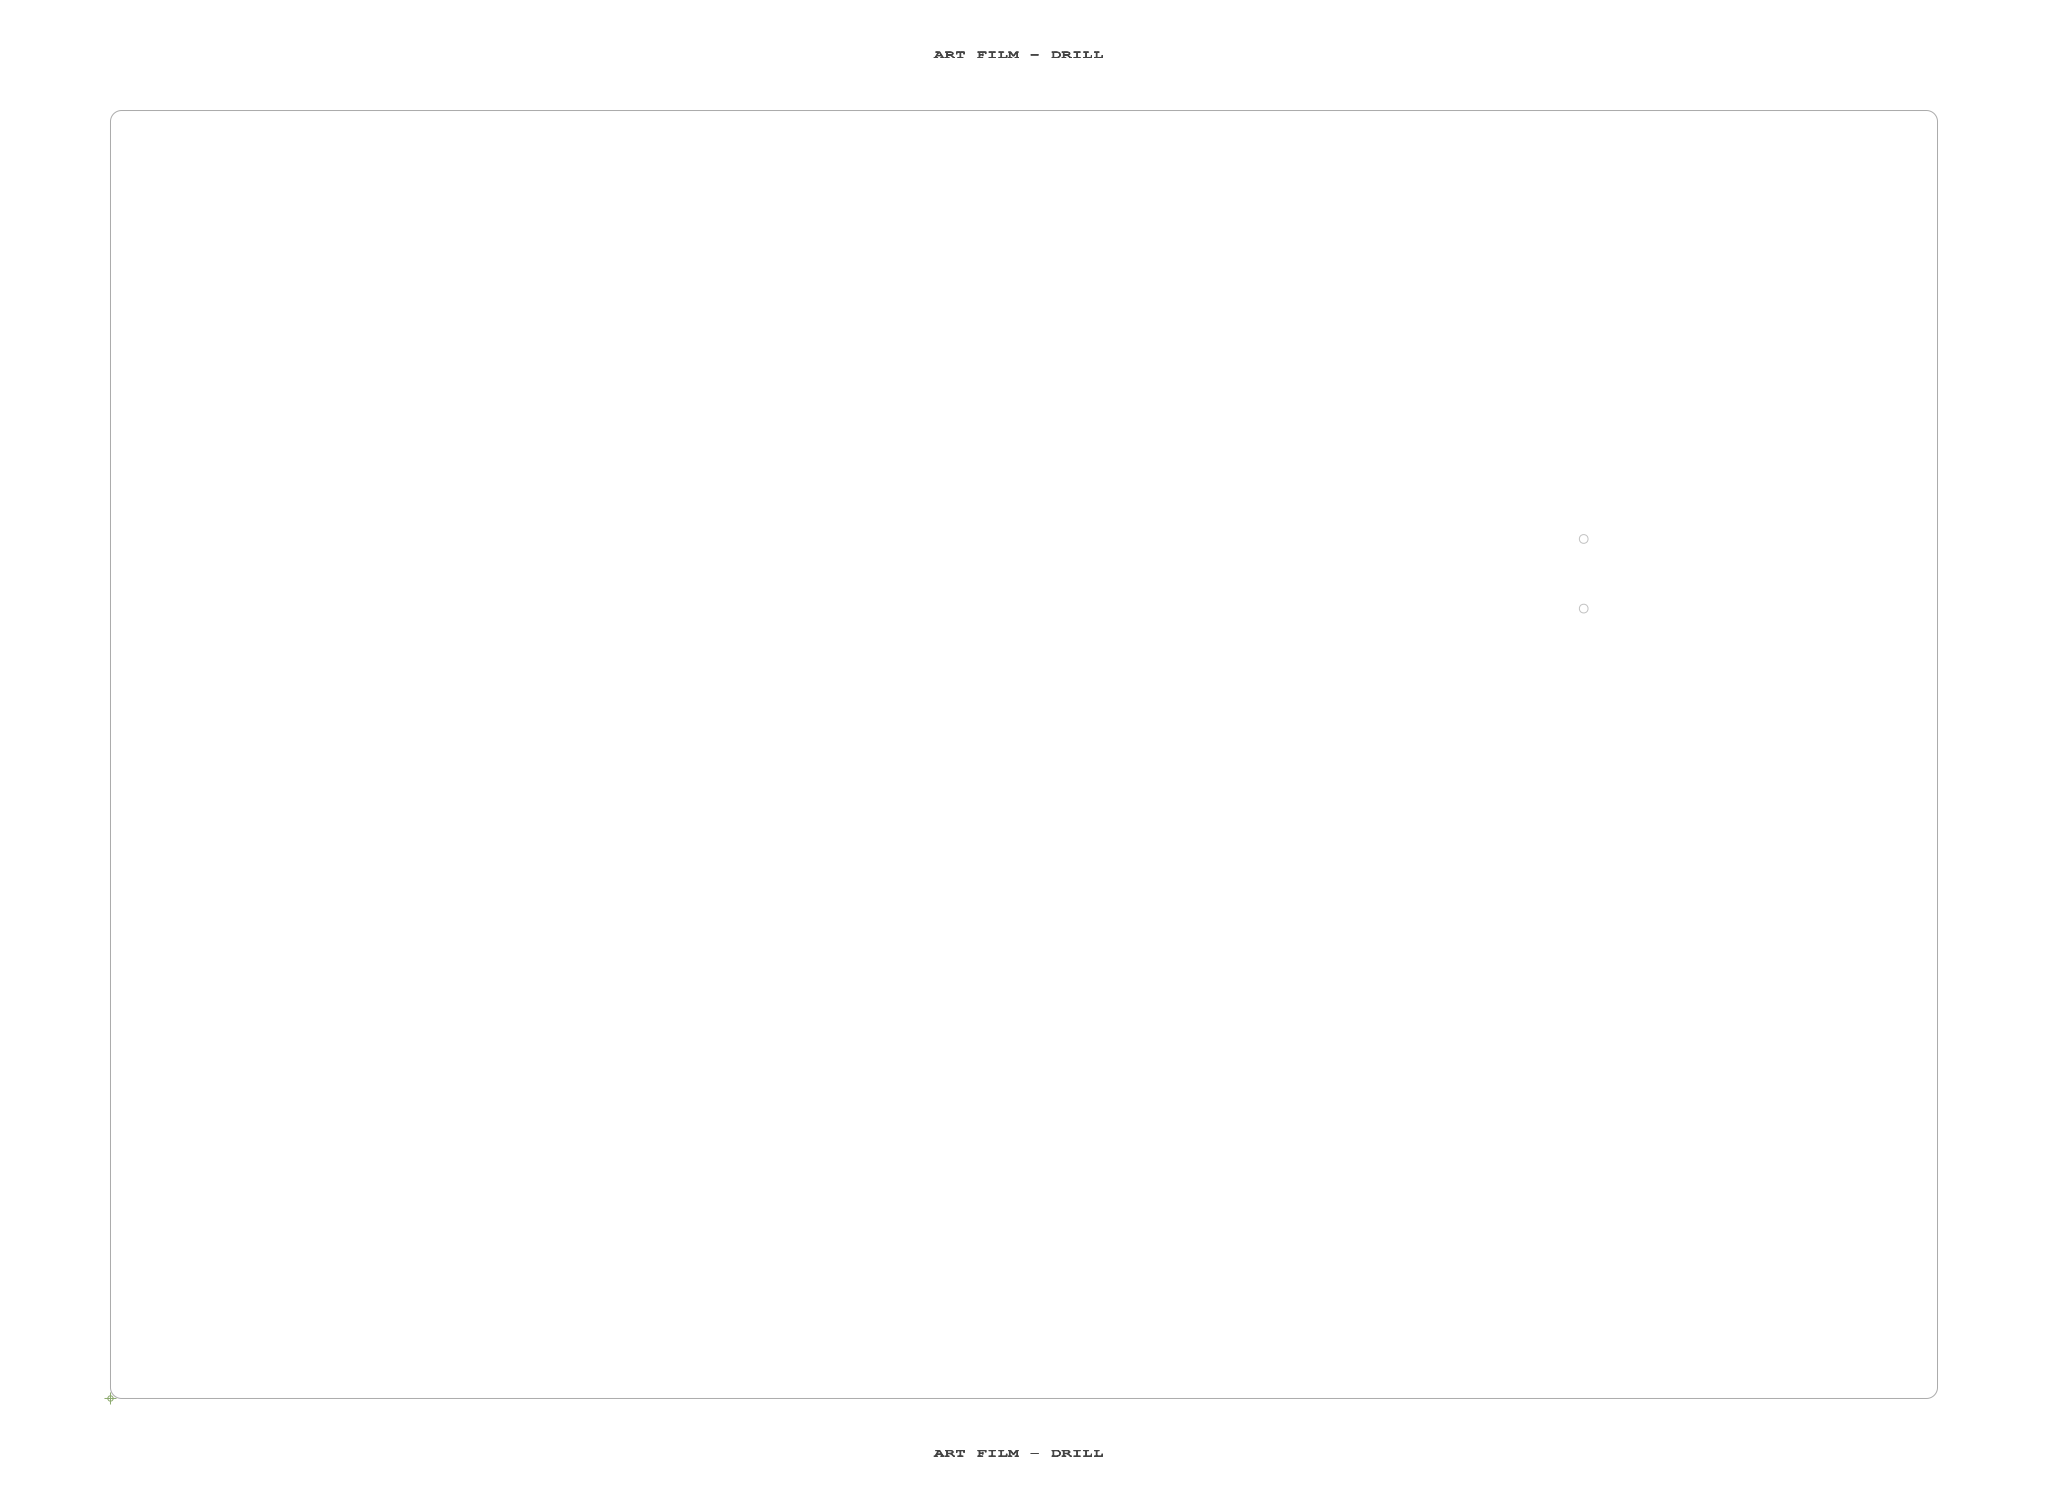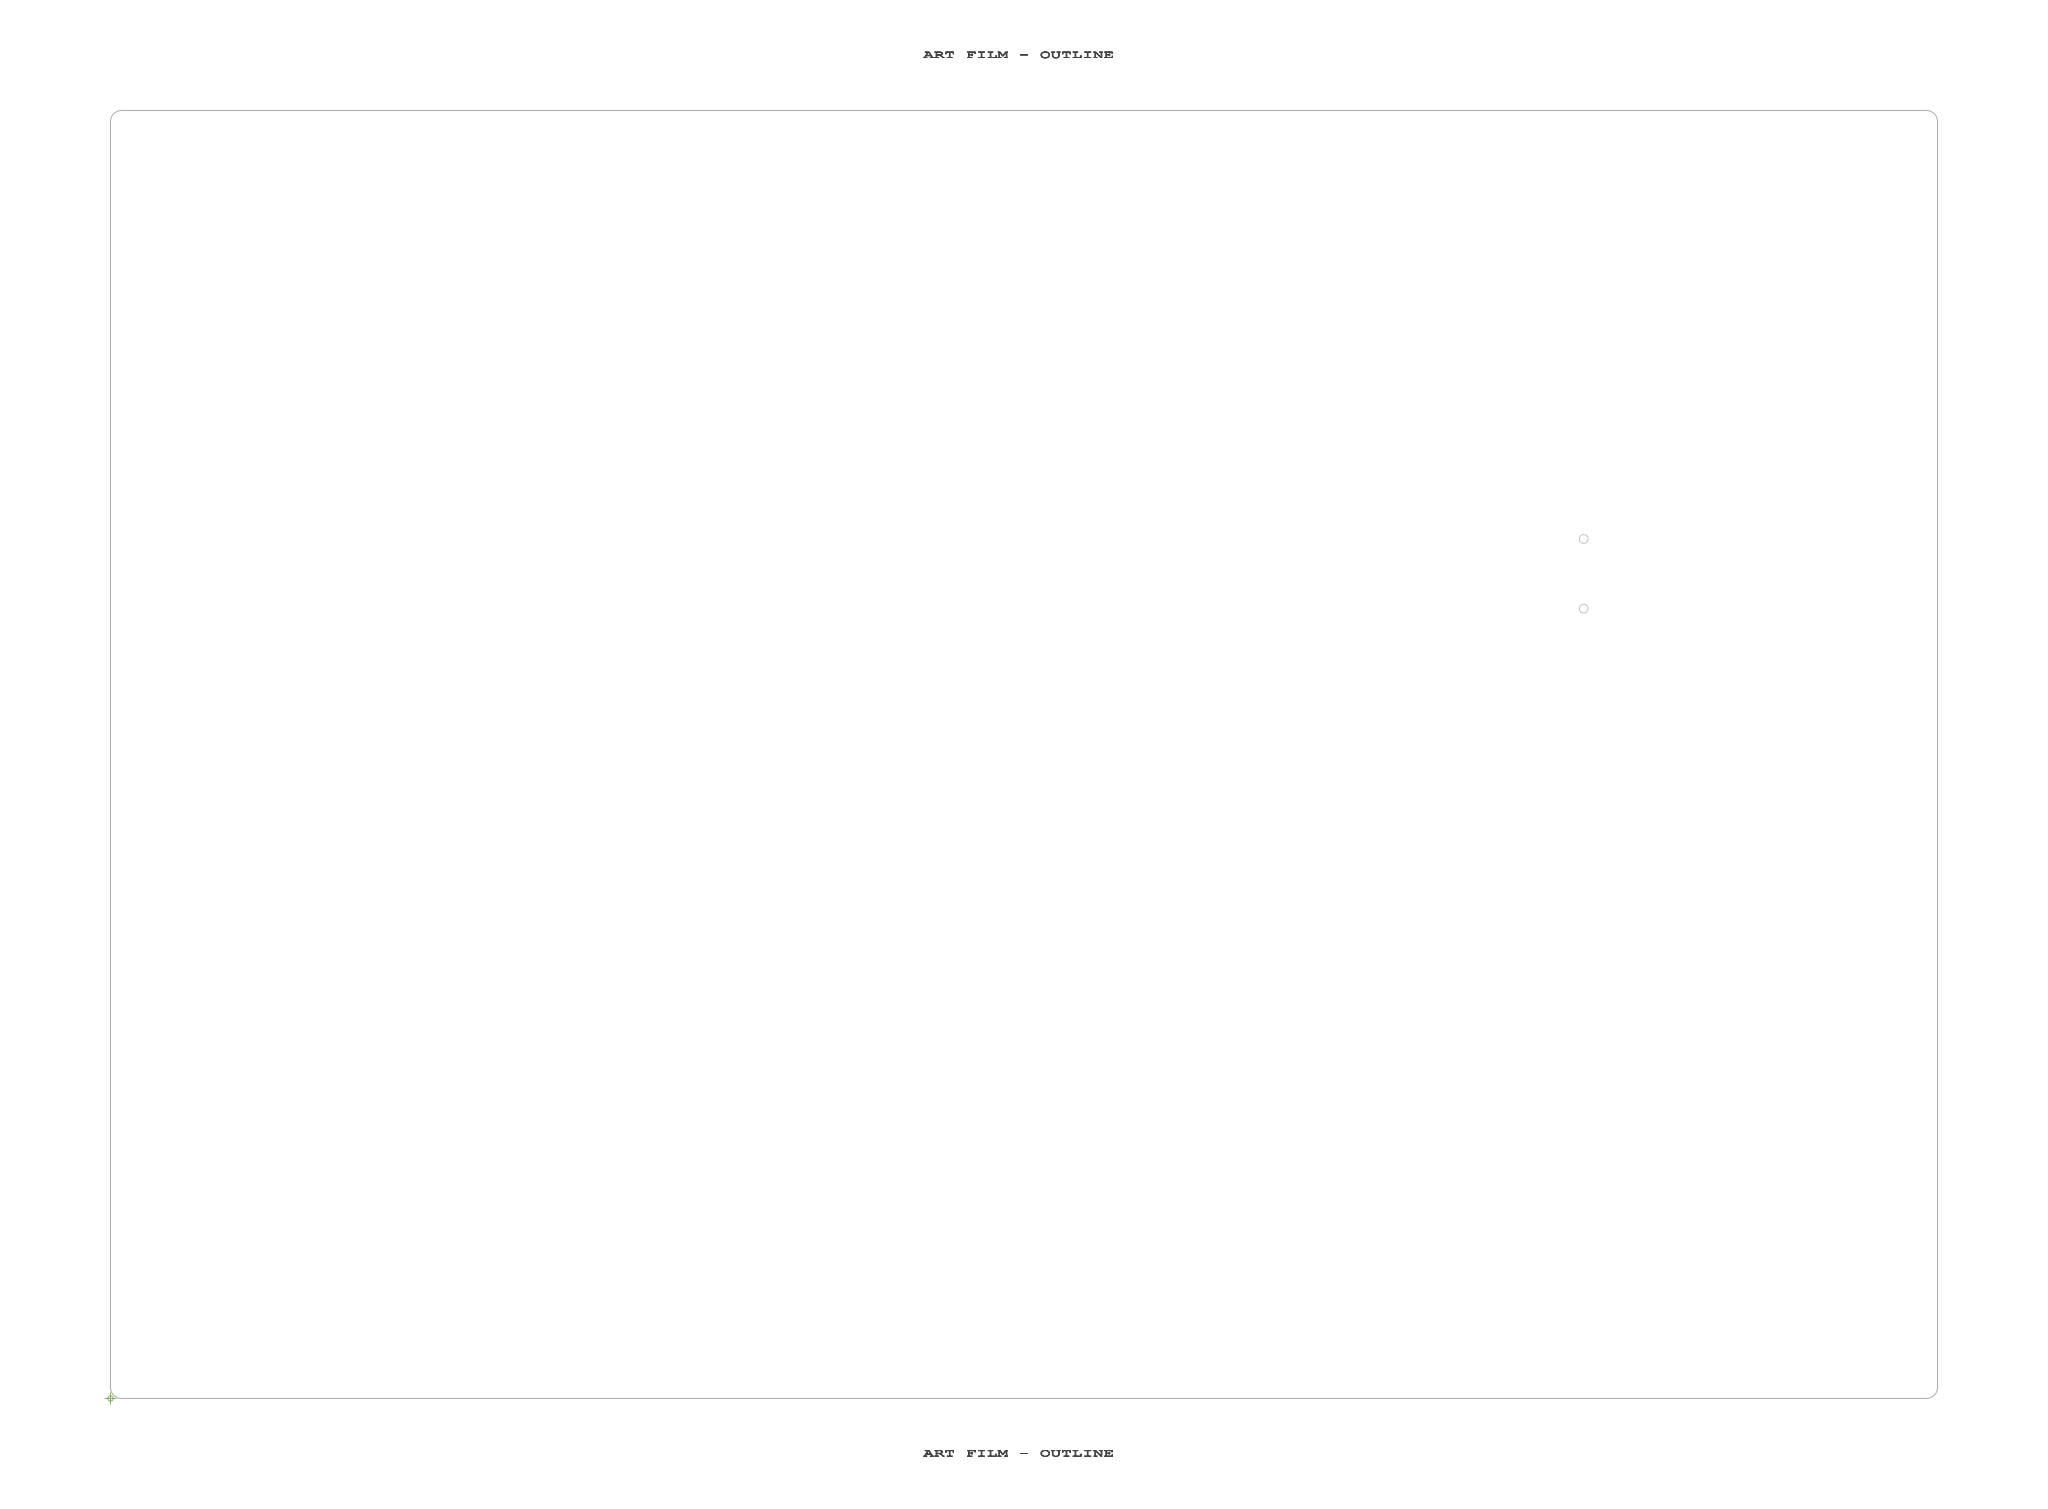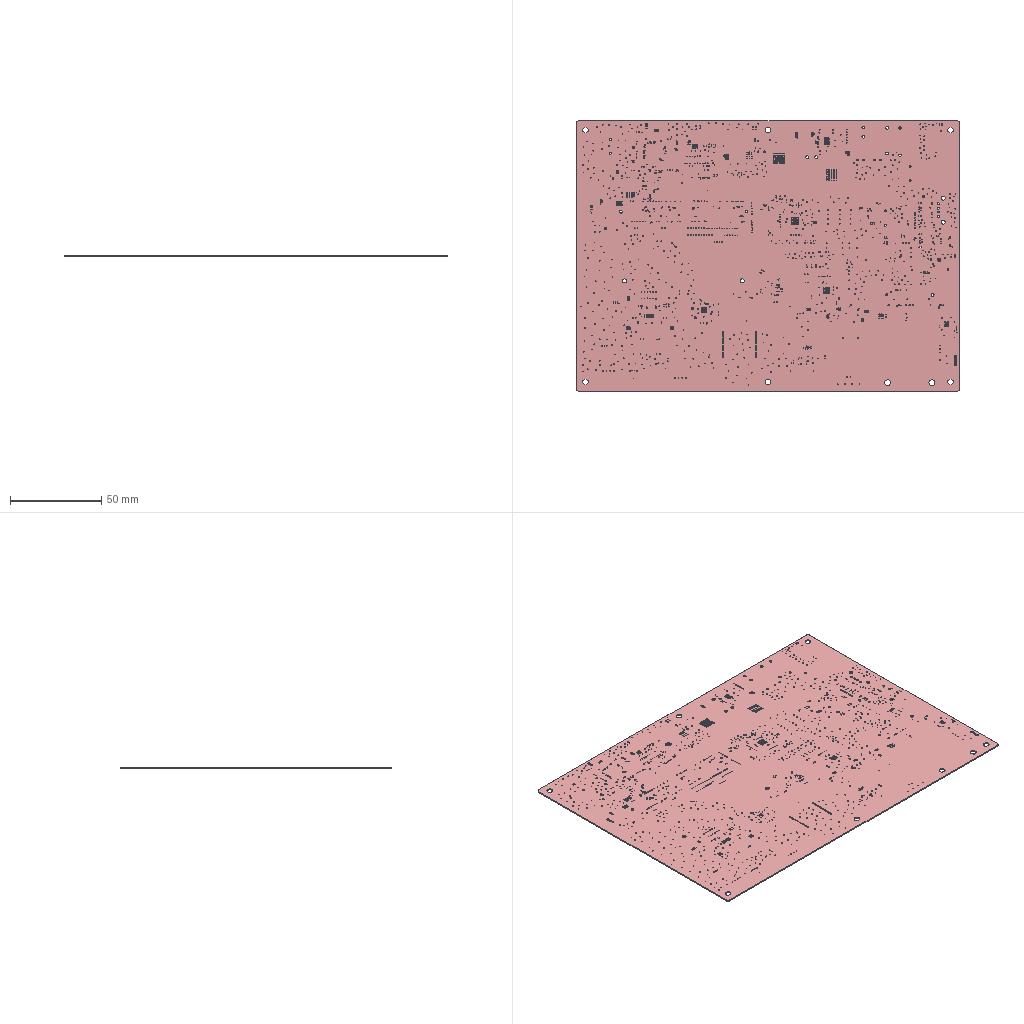Circuit board layout | Cadence Allegro | box 210 x 148 x 0.7 mm
Layer stack:
# Cadence Allegro layer stack of  (unit mm; from the constraint file cross-section; dielectric type: 0 not recorded (Allegro does not mark core vs prepreg), 3 surface material)
index,name,kind,layer,copper_thickness_mm,dielectric_type,dielectric_thickness_mm,dielectric_material,dielectric_constant
0,Top Surface,other,,,,,,
1,TOP,copper,TOP,0.0305,,,,
2,Dielectric1,dielectric,,,0,0.2032,FR-4,4.5
3,GND2,copper,GND2,0.0305,,,,
4,Dielectric2,dielectric,,,0,0.2032,FR-4,4.5
5,VCC3,copper,VCC3,0.0305,,,,
6,Dielectric3,dielectric,,,0,0.2032,FR-4,4.5
7,BOTTOM,copper,BOTTOM,0.0305,,,,
8,Bottom Surface,other,,,,,,
# drill layer pairs: low layer,high layer
drill_pair,TOP,BOTTOM
Part placement, first 550 of 616 lines:
REFDES,COMP_VALUE,SYM_NAME,SYM_X,SYM_Y,SYM_ROTATE,SYM_MIRROR
BT1,3V BAT,BAT600,731.008,5280.740,180.000,NO
C1,0.1uF/275V,C_18X6L,6981.850,5380.748,270.000,NO
C2,100nF,C0603,6496.929,4878.504,0.000,YES
C3,100nF,C0603,4264.664,5392.967,270.000,NO
C4,100nF,C0603,5492.165,5274.055,0.000,YES
C5,100nF,C0603,5766.479,5354.193,0.000,NO
C6,1uF,C0603,5278.819,5296.654,270.000,YES
C7,1uF,C0603,5765.731,5530.531,0.000,YES
C8,330pF,C0603,5767.402,5586.993,0.000,NO
C9,100nF,C0603,5768.303,5644.372,0.000,NO
C10,10nF,C0603,5462.622,5634.250,0.000,NO
C11,100nF,C0603,4031.414,5277.712,0.000,YES
C12,10uF/16V,C1206,3986.867,5314.380,180.000,NO
C13,2.2nF,C0603,5462.898,5566.801,0.000,NO
C14,1uF,C0603,5279.173,5424.528,90.000,YES
C15,10uF/16V,C1206,2817.520,5683.311,180.000,NO
C16,100nF,C0603,2558.740,5380.433,270.000,YES
C17,100nF,C0603,3352.205,5043.366,180.000,YES
C18,10uF/16V,C1206,3708.783,5592.795,90.000,NO
C19,10uF/16V,C1206,4892.301,1037.077,270.000,NO
C20,100nF,C0603,8083.170,1525.692,270.000,YES
C21,1nF,C0603,3502.319,4768.850,270.000,NO
C22,100nF,C0603,5241.942,1678.011,0.000,YES
C23,100nF,C0603,8202.820,1450.328,90.000,NO
C24,10uF/16V,C1206,7896.426,1719.824,90.000,NO
C25,100nF,C0603,3330.071,4721.878,180.000,YES
C26,100nF,C0603,8156.690,1222.130,90.000,YES
C27,100nF,C0603,4826.647,1609.621,90.000,NO
C28,100nF,C0603,5423.307,2711.417,90.000,YES
C29,100nF,C0603,5511.377,2212.857,270.000,YES
C30,22pF/50V,C0603,4973.224,2384.386,0.000,YES
C31,100nF,C0603,706.654,4602.992,0.000,NO
C32,22pF/50V,C0603,4962.673,2473.283,180.000,YES
C33,1nF,C0603,832.638,4595.157,270.000,YES
C34,100nF,C0603,937.205,4611.535,90.000,YES
C35,1uF/16V,C0603,5141.297,2057.270,180.000,NO
C36,1uF/16V,C0603,5586.850,2194.449,90.000,NO
C37,100nF,C0603,5296.181,2405.748,270.000,YES
C38,100nF,C0603,1123.346,4574.764,180.000,YES
C39,100nF,C0603,1465.315,4392.087,0.000,YES
C40,100nF,C0603,1485.709,4491.969,180.000,YES
C41,10uF/6.3V,C0805,1745.787,4651.279,0.000,NO
C42,100nF,C0603,1742.637,4568.602,0.000,NO
C43,10uF/6.3V,C0805,5154.232,3379.386,270.000,NO
C44,100nF,C0603,5037.118,3353.618,0.000,NO
C45,100nF,C0603,4741.547,3437.087,270.000,NO
C46,22pF/50V,C0603,5004.016,3745.902,180.000,YES
C47,100nF,C0603,4684.720,3436.811,270.000,NO
C48,100nF,C0603,4704.346,3554.295,0.000,YES
C49,100nF,C0603,4832.500,3736.449,270.000,YES
C50,100nF,C0603,4840.000,3875.000,180.000,YES
C51,22pF/50V,C0603,5015.236,3655.579,0.000,YES
C52,100nF,C0603,5159.031,3880.701,180.000,YES
C53,1uF/16V,C0603,5021.559,3880.874,0.000,NO
C54,100nF,C0603,4720.409,3790.437,0.000,YES
C55,100nF,C0603,4830.224,3604.929,90.000,YES
C56,10uF/6.3V,C0805,4690.162,4062.890,180.000,NO
C57,100nF,C0603,3620.700,2111.190,90.000,NO
C58,1nF/2kV,C1206,8054.163,483.534,0.000,YES
C59,100nF,C0603,3863.570,2117.570,270.000,NO
C60,100nF,C0603,3425.640,2116.160,270.000,NO
C61,100nF,C0603,2841.681,1765.520,90.000,YES
C62,100nF,C0603,2761.866,1843.043,0.000,YES
C63,4.7uF/16V,C0603,2531.024,1674.752,180.000,NO
C64,4.7uF/16V,C0603,2681.594,1535.354,270.000,NO
C65,4.7uF/16V,C0603,2821.295,1535.118,270.000,NO
C66,100nF,C0603,805.075,1990.827,90.000,NO
C67,4.7uF/16V,C0603,2741.634,1535.354,270.000,NO
C68,4.7uF/16V,C0603,2993.740,1643.618,0.000,NO
C69,1uF/16V,C0603,2989.008,1760.673,180.000,NO
C70,1nF,C0603,1945.232,1503.882,270.000,YES
C71,100nF,C0603,1878.988,1503.898,270.000,YES
C72,1uF/16V,C0603,1663.343,1897.094,270.000,NO
C73,220nF,C0603,1792.870,1359.024,270.000,NO
C74,330pF,C0603,1789.287,1181.031,270.000,NO
C75,1nF,C0603,1789.413,1049.197,90.000,NO
C76,1nF/50V,C0603,1723.972,1898.354,270.000,NO
C77,1uF/16V,C0603,1609.091,1897.488,270.000,NO
C78,4.7uF/16V,C0603,1719.201,2068.079,270.000,YES
C79,220nF,C0603,1623.618,1355.323,270.000,NO
C80,1nF,C0603,1734.728,1048.094,90.000,NO
C81,330pF,C0603,1735.823,1181.031,270.000,NO
C82,220nF,C0603,1567.831,1355.323,270.000,NO
C83,330pF,C0603,1450.469,1185.756,270.000,NO
C84,1nF,C0603,1452.051,1054.276,90.000,NO
C85,1uF/16V,C0603,1513.264,1896.780,270.000,NO
C86,1uF/16V,C0603,1457.122,1896.543,270.000,NO
C87,1uF/16V,C0603,1544.717,1921.264,180.000,YES
C88,1nF/50V,C0603,1342.476,1897.220,270.000,NO
C89,220nF,C0603,1449.209,1356.110,270.000,NO
C90,330pF,C0603,1380.043,1183.598,270.000,NO
C91,1nF,C0603,1379.106,1050.071,90.000,NO
C92,1uF/16V,C0603,1431.937,1737.343,180.000,YES
C93,1nF,C0603,1219.799,1513.606,270.000,YES
C94,100nF,C0603,1279.894,1513.709,270.000,YES
C95,33pF/50V,C0603,7113.106,3118.780,270.000,YES
C96,100nF,C0603,7175.681,3118.850,270.000,YES
C97,33pF/50V,C0603,6956.102,2988.902,180.000,YES
C98,100nF,C0603,7138.307,1914.105,0.000,YES
C99,100nF,C0603,7613.897,1911.428,0.000,YES
C100,100nF,C0603,6869.960,2233.869,0.000,YES
C101,100nF,C0603,6755.141,1908.688,180.000,YES
C102,10nF,C0603,5697.516,1596.142,270.000,YES
C103,100nF,C0603,5526.008,1662.587,180.000,YES
C104,100nF,C0603,3785.917,907.630,270.000,YES
C105,10uF/16V,C1206,1650.567,5698.067,0.000,NO
C106,10uF/16V,C1206,1853.579,4869.008,270.000,NO
C107,4.7uF/25V,C0805,1879.142,5700.106,180.000,NO
C108,4.7uF/25V,C0805,2117.413,4867.835,270.000,NO
C109,100nF,C0603,1999.850,5406.547,0.000,YES
C110,10nF,C0603,1979.134,5538.587,180.000,NO
C111,100nF,C0603,1862.252,5173.240,0.000,YES
C112,4.7uF/50V,C1206,2290.661,5366.169,180.000,NO
C113,10nF,C0603,1979.843,5102.791,0.000,NO
C114,4.7uF/50V,C1206,2302.827,5215.854,180.000,NO
C115,4.7uF/25V,C0805,1585.909,5528.016,270.000,NO
C116,4.7uF/25V,C0805,1355.740,5247.744,180.000,NO
C117,4.7uF/25V,C0805,1489.689,5528.016,270.000,NO
C118,4.7uF/25V,C0805,1356.000,5248.000,180.000,YES
C119,10uF/16V,C1206,1344.528,4955.157,0.000,NO
C120,4.7uF/16V,C0603,1374.701,5110.484,180.000,NO
C121,4.7uF/16V,C0603,1371.339,5383.272,180.000,NO
C122,4.7uF/16V,C0603,1494.839,4918.110,270.000,YES
C123,4.7uF/25V,C0805,1575.169,4894.008,270.000,NO
C124,4.7uF/16V,C0603,1631.811,5311.933,180.000,YES
C125,10uF/16V,C1206,632.165,3631.685,270.000,NO
C126,100nF,C0603,628.453,3661.850,90.000,YES
C127,10uF/50V,C1210,524.189,3838.185,180.000,NO
C128,10uF/50V,C1210,524.173,3976.728,180.000,NO
C129,100nF,C0603,494.740,4005.311,0.000,YES
C130,100nF,C0603,810.108,507.362,90.000,NO
C131,100nF,C0603,653.701,1042.756,270.000,YES
C132,1nF,C0603,1900.323,641.807,0.000,NO
C133,100nF,C0603,1726.878,722.055,90.000,YES
C134,100nF,C0603,1140.933,506.606,90.000,NO
C135,10nF,C0603,1255.508,507.047,270.000,NO
C136,100nF,C0603,6186.646,3883.374,180.000,YES
C137,10uF/16V,C1206,6377.287,3762.906,90.000,YES
C138,100nF,C0603,7724.043,2838.444,180.000,NO
C139,10uF/16V,C1206,7531.311,2715.312,270.000,NO
C140,100nF,C0603,7362.551,2690.584,180.000,NO
C141,4.7uF/16V,C0603,4271.159,2003.369,90.000,YES
C142,100nF,C0603,4328.583,2002.771,90.000,YES
C143,4.7uF/16V,C0603,4326.497,2372.333,270.000,YES
C144,100nF,C0603,4384.819,2372.591,270.000,YES
C145,100nF,C0603,4165.028,2336.150,90.000,YES
C146,100nF,C0603,6991.626,3764.244,270.000,YES
C147,100nF,C0603,5291.024,586.505,0.000,NO
C148,100nF,C0603,4910.492,607.698,270.000,YES
C149,100nF,C0603,5029.583,604.419,0.000,YES
C150,100nF,C0603,5290.394,642.608,0.000,NO
C151,100nF,C0603,5030.181,706.151,0.000,YES
C152,100nF,C0603,4497.315,750.812,180.000,YES
CE1,100uF/50V,CE8X11D5P3D5L,6564.961,4988.110,180.000,NO
CE2,100uF/50V,CE8X11D5P3D5L,6197.677,4988.110,180.000,NO
CE3,470uF/16V,CE8X11D5P3D5L,4060.489,5162.845,180.000,NO
CN1,SIM CARD,SIMCARD-6P-A,6640.000,2940.000,0.000,NO
CT1,100uF/10V,B_CASE,2555.358,5463.669,90.000,NO
CT2,470uF/10V,E_CASE,3342.559,5042.949,0.000,NO
CT3,470uF/10V,E_CASE,5271.423,1641.286,180.000,NO
CT4,100uF/16V,D_CASE,1911.461,1609.386,90.000,NO
CT5,100uF/16V,D_CASE,1251.736,1627.654,90.000,NO
CT6,470uF/10V,E_CASE,6419.654,1896.765,270.000,NO
CT7,100uF/10V,B_CASE,5698.390,1625.220,90.000,NO
D1,5KP48CA,5KP48A,6705.827,5400.433,90.000,NO
D2,BZT52C15,SOD-123FL,7158.031,5155.433,90.000,YES
D3,MBRD1045T4G,SOT428,4370.588,4836.703,0.000,NO
D4,MBRD1045T4G,SOT428,5687.520,4663.386,90.000,NO
D5,B340A,DO-214AA,3709.409,5303.945,180.000,NO
D6,B340A,DO-214AA,5115.186,1019.463,90.000,NO
D7,B340A,DO-214AA,8079.625,1735.726,180.000,NO
D8,MBR140SFT1,SOD-123FL,747.913,4718.504,0.000,NO
D9,MBR140SFT1,SOD-123FL,576.142,4591.496,90.000,NO
D10,ESDA,0603ESDA,2919.882,528.193,180.000,NO
D11,0603ESDA,0603ESDA,7049.646,3122.445,180.000,YES
D12,0603ESDA,0603ESDA,7104.563,2936.575,270.000,YES
D13,0603ESDA,0603ESDA,7104.760,2831.575,270.000,YES
D14,0603ESDA,0603ESDA,6176.736,2829.213,90.000,YES
D15,MBR140SFT1,SOD-123FL,1827.886,5514.512,90.000,NO
D16,MBR140SFT1,SOD-123FL,1978.583,5017.020,0.000,NO
D17,BAS70-04,SOT23,2009.846,5208.559,270.000,NO
D18,BAS70-04,SOT23,2013.114,5369.346,270.000,NO
D19,B340A,DO-214AA,170.394,3938.339,180.000,NO
D20,ESDA,0603ESDA,1872.874,521.185,180.000,NO
D21,ESDA,0603ESDA,7599.642,4081.412,270.000,YES
D22,ESDA,0603ESDA,7599.681,4025.884,270.000,YES
D23,ESDA,0603ESDA,7798.161,3285.891,270.000,YES
D24,ESDA,0603ESDA,7797.768,3231.214,270.000,NO
D25,ESDA,0603ESDA,7797.791,3176.844,270.000,NO
D26,ESDA,0603ESDA,7600.358,3917.869,90.000,NO
D27,ESDA,0603ESDA,7600.083,3746.436,90.000,NO
D28,ESDA,0603ESDA,7627.500,3189.930,90.000,YES
D29,ESDA,0603ESDA,7626.949,3297.505,90.000,YES
D30,ESDA,0603ESDA,7626.949,3243.647,90.000,YES
D31,0603ESDA,0603ESDA,5288.390,756.572,270.000,YES
D32,0603ESDA,0603ESDA,4759.579,660.982,90.000,YES
D33,0603ESDA,0603ESDA,5289.177,700.509,270.000,YES
D34,0603ESDA,0603ESDA,4760.169,605.549,90.000,YES
F1,FUSE 4A 125V,F_065,7479.819,4714.008,0.000,NO
FB1,60R,FB0603,5154.610,3548.567,270.000,NO
FB2,60R,FB0603,4745.713,3927.984,90.000,NO
FB3,60R,FB0603,2531.283,1741.201,0.000,NO
FB4,60R,FB0603,2883.823,1533.346,90.000,NO
FB5,60R,FB0603,2849.484,524.173,270.000,NO
FB6,220R 2A,FB0805,1930.354,1356.350,0.000,NO
FB7,220R 2A,FB0805,1869.563,1139.031,270.000,NO
FB8,220R 2A,FB0805,1648.854,1137.654,270.000,NO
FB9,220R 2A,FB0805,1539.909,1136.551,270.000,NO
FB10,220R 2A,FB0805,1293.587,1138.724,270.000,NO
FB11,220R 2A,FB0805,1245.118,1366.358,180.000,NO
FB12,60R,FB0603,1802.319,517.063,270.000,NO
H1,PM,MH_3P2MM,196.850,196.850,0.000,NO
H2,PM,MH_3P2MM,4133.858,196.850,0.000,NO
H3,PM,MH_3P2MM,8070.866,196.850,0.000,NO
H4,PM,MH_3P2MM,4133.858,5629.921,0.000,NO
H5,PM,MH_3P2MM,8070.866,5629.921,0.000,NO
H6,PM,MH_3P2MM,196.850,5629.921,0.000,NO
J1,2pin_2mm_CR,PBV2_200,7930.157,5142.717,270.000,NO
J2,3pin_2mm_CR,PBV3_200,7933.610,2691.240,270.000,NO
J3,SAIL_i.MX7D,DDR4_SLT_RVS,958.189,3871.496,180.000,NO
J4,6pin_2mm_CR,PBV6_200,7920.737,986.112,270.000,NO
J5,3pin_2mm_CR,PBV3_200,2849.567,354.646,180.000,NO
J6,4pin_2mm_CR,PBV4_200,2364.173,354.646,180.000,NO
J7,ZIF_FPC_39pin,39FXL,2413.386,4810.039,180.000,YES
J8,6pin_0.5mm_FPC,6PIN_05MM_FPC_UP,275.591,4419.291,180.000,YES
J9,4pin_2mm_CR,PBV4_200,810.394,353.189,180.000,NO
J10,3pin_2mm_CR,PBV3_200,1802.835,354.646,180.000,NO
J11,3pin_2mm_CR,PBV3_200,1313.465,354.646,180.000,NO
J12,Mini-USB-B,MINI_USB_B,8082.968,3220.284,90.000,NO
J13,Mini-USB_DIP,MICRO_USB_BS,7399.900,3867.550,90.000,NO
J14,Mini-USB_DIP,MICRO_USB_BS,7411.260,3193.660,90.000,NO
J15,TF_SOCKET,TF_001,7085.000,3605.000,270.000,NO
J16,3pin_2mm_CR,PBV3_200,5274.961,350.433,180.000,NO
J17,5pin_2mm_CR,PBV5_200,4777.323,349.213,180.000,NO
L1,10uH_NC,IND_VLS6045,6200.000,5250.197,0.000,NO
L2,10uH,L_C150_C50,6191.772,5389.961,90.000,NO
L3,10uH_NC,IND_VLS6045,4754.350,5046.063,270.000,NO
L4,10uH,L_C150_C50,4879.232,5044.330,0.000,NO
L5,22uH,IND_VLS6045,3428.740,5296.949,0.000,NO
L6,22uH,IND_VLS6045,5198.686,1337.148,270.000,NO
L7,4.7uH,IND_VLS3012_SM,5007.008,3465.008,270.000,NO
L8,2.2uH,IND_VLS3012_SM,1709.882,5511.134,270.000,NO
L9,4.7uH,IND_VLS3012_SM,1989.260,4865.748,270.000,NO
L10,22uH,IND_VLS6045,201.823,3597.157,270.000,NO
LED1,GREEN,LED0805,5675.465,3335.862,180.000,NO
LED2,GREEN,LED0805,5673.622,3440.902,180.000,NO
LED3,GREEN,LED0805,4534.941,3963.575,270.000,NO
LED4,GREEN,LED0805,4424.705,3963.811,270.000,NO
LED5,GREEN,LED0805,5650.748,2947.067,0.000,NO
LED6,GREEN,LED0805,5653.260,2839.421,0.000,NO
Q1,BUK7226-75A,SOT428,7718.504,5500.157,180.000,NO
Q2,SQD50N06-07L,SOT428,4495.781,5437.175,0.000,NO
Q3,SI4856ADY,SOIC8,4927.273,5541.570,90.000,NO
Q4,S9014,SOT23,8028.613,1236.745,270.000,NO
Q5,S9014,SOT23,4692.874,1623.741,180.000,YES
Q6,AO3401,SOT23,1002.965,1984.984,270.000,NO
Q7,S9014,SOT23,651.909,1985.724,270.000,NO
Q8,S9014,SOT23,7198.511,1711.144,0.000,YES
Q9,AO3401,SOT23,5526.827,1540.350,180.000,NO
Q10,S9014,SOT23,5454.098,1765.226,270.000,NO
Q11,S9014,SOT23,2912.012,849.780,270.000,NO
Q12,S9014,SOT23,1234.827,689.059,0.000,NO
Q13,AO3401,SOT23,7370.331,2817.206,0.000,NO
Q14,S9015,SOT23,4236.323,826.647,180.000,NO
R1,5.1K,R0805,7156.614,5630.709,270.000,YES
R2,1R00,R0805,5736.299,5272.835,0.000,NO
R3,75K 1%,R0603,5766.125,5413.708,0.000,NO
R4,1M,R0603,5765.731,5530.531,0.000,NO
R5,29.4K 1%,R0603,5766.440,5413.748,0.000,YES
R6,16.2K 1%,R0603,5765.849,5470.334,180.000,NO
R7,10K,R0603,5492.827,5602.496,270.000,YES
R8,0R 1%,R0603,5324.453,5106.898,0.000,NO
R9,13K 1%,R0603,5320.814,5566.960,0.000,NO
R10,R020,R2512,5511.260,5017.677,270.000,NO
R11,R020,R2512,5725.354,5017.677,270.000,NO
R12,0R 1%,R0603,5323.508,5183.906,0.000,NO
R13,1.47K 1%,R0603,5320.814,5632.826,180.000,NO
R14,13K 1%,R0603,3440.276,5645.768,0.000,YES
R15,40.2K 1%,R0603,3331.579,5614.071,90.000,YES
R16,13K 1%,R0603,4891.619,1442.727,180.000,YES
R17,29.4K 1%,R0603,5023.060,1442.294,180.000,YES
R18,620K,R0603,3623.280,4768.992,270.000,NO
R19,100K,R0603,4892.671,1609.290,90.000,NO
R20,39K,R0603,3564.799,4768.677,270.000,NO
R21,10K,R0603,8156.744,1222.375,270.000,NO
R22,90.9K 1%,R0603,7882.249,1514.101,270.000,YES
R23,10K,R0603,4684.527,1824.788,0.000,YES
R24,4.7K,R0603,7880.952,1245.194,270.000,NO
R25,4.7K,R0603,4684.260,1752.292,180.000,YES
R26,13K 1%,R0603,7883.289,1386.164,270.000,YES
R27,10K,R0603,5356.102,2712.323,90.000,YES
R28,22R,R0603,5423.307,2712.323,270.000,NO
R29,1K_NC,R0603,1258.728,3441.630,90.000,YES
R30,1K,R0603,5689.213,3338.106,180.000,YES
R31,1K_NC,R0603,1319.280,3442.024,90.000,YES
R32,0R,R0603,2593.000,3917.000,0.000,YES
R33,1K,R0603,5686.701,3439.051,180.000,YES
R34,1K,R0603,5809.512,3089.374,0.000,YES
R35,1K,R0603,5809.748,3189.256,0.000,YES
R36,0R_NC,R0603,707.047,4521.693,0.000,NO
R37,10K,R0603,3309.055,3432.913,90.000,YES
R38,10K,R0603,3364.409,3432.992,90.000,YES
R39,10K,R0603,3418.307,3432.913,90.000,YES
R40,100K,R0603,575.354,4597.559,270.000,YES
R41,10K,R0603,3472.047,3432.362,90.000,YES
R42,0R_NC,R0603,5750.591,3605.433,180.000,YES
R43,0R_NC,R0603,5750.591,3705.236,180.000,YES
R44,0R_NC,R0603,5750.591,3806.811,180.000,YES
R45,0R_NC,R0603,5750.591,3905.669,180.000,YES
R46,10K,R0603,2866.220,3434.528,90.000,YES
R47,10K,R0603,2922.717,3434.528,90.000,YES
R48,620K,R0603,687.795,4593.661,90.000,YES
R49,10K,R0603,2978.268,3278.346,90.000,YES
R50,4.7K,R0603,2978.307,3434.173,90.000,YES
R51,10K,R0603,3033.449,3278.386,90.000,YES
R52,4.7K,R0603,3033.819,3433.937,90.000,YES
R53,10K,R0603,3089.055,3278.386,90.000,YES
R54,4.7K,R0603,3089.055,3433.622,90.000,YES
R55,10K,R0603,3143.252,3279.331,90.000,YES
R56,4.7K,R0603,3143.701,3433.543,90.000,YES
R57,10K,R0603,3198.228,3432.992,90.000,YES
R58,10K,R0603,3253.622,3432.992,90.000,YES
R59,10K,R0603,2410.866,3436.063,90.000,YES
R60,10K,R0603,2467.677,3436.063,90.000,YES
R61,12K 1%,R0603,5141.524,1998.090,180.000,NO
R62,100K,R0603,5418.543,2405.748,270.000,NO
R63,100K,R0603,5356.929,2405.748,270.000,NO
R64,10K,R0603,2525.394,3435.748,90.000,YES
R65,10K,R0603,2582.205,3435.748,90.000,YES
R66,10K,R0603,2639.646,3435.472,90.000,YES
R67,10K,R0603,2696.772,3435.157,90.000,YES
R68,10K,R0603,2753.858,3434.843,90.000,YES
R69,10K,R0603,2810.315,3434.488,90.000,YES
R70,100K,R0603,5296.181,2405.315,90.000,NO
R71,100K,R0603,5238.976,2405.787,90.000,NO
R72,100K,R0603,5477.559,2405.787,90.000,NO
R73,4.7K,R0603,1245.354,4681.693,90.000,NO
R74,4.7K,R0603,1185.512,4682.598,90.000,NO
R75,4.7K,R0603,1686.535,4430.512,270.000,YES
R76,4.7K,R0603,1750.039,4430.512,270.000,YES
R77,10K,R0603,1474.016,4566.063,0.000,NO
R78,10K,R0603,4466.339,3645.287,0.000,NO
R79,1.5K,R0603,4798.768,3435.724,90.000,NO
R80,10K,R0603,4857.657,3434.874,270.000,NO
R81,10K_NC,R0603,4466.000,3645.335,180.000,YES
R82,10K,R0603,4466.260,3698.437,0.000,NO
R83,10K,R0603,4687.736,3927.984,270.000,NO
R84,10K,R0603,4466.142,3589.146,0.000,NO
R85,10K,R0603,4466.102,3753.240,0.000,NO
R86,10K,R0603,4466.102,3533.043,0.000,NO
R87,10K,R0603,5000.669,3582.075,0.000,NO
R88,10K,R0603,4629.051,3434.543,270.000,NO
R89,10K,R0603,4465.906,3809.343,0.000,NO
R90,10K,R0603,4631.043,3928.811,270.000,NO
R91,0R_NC,R0603,4932.398,3492.063,90.000,YES
R92,1K,R0603,4535.571,3989.016,270.000,YES
R93,2.37K 1%,R0603,5020.945,3822.319,180.000,NO
R94,1K,R0603,4424.862,3988.701,270.000,YES
R95,0R,R0603,5021.583,3880.626,180.000,YES
R96,49.9R 1%,R0603,3797.709,2116.953,90.000,NO
R97,49.9R 1%,R0603,3740.308,2116.874,90.000,NO
R98,49.9R 1%,R0603,3548.764,2115.415,90.000,NO
R99,49.9R 1%,R0603,3490.378,2115.510,90.000,NO
R100,75R 1%,R0603,3697.140,1559.990,180.000,YES
R101,75R 1%,R0603,8080.879,749.660,180.000,YES
R102,75R 1%,R0603,8080.879,592.100,180.000,YES
R103,47K,R0603,872.154,1990.685,90.000,NO
R104,39K,R0603,2993.795,1702.476,0.000,YES
R105,0R_NC,R0603,2993.819,1702.303,0.000,NO
R106,10K,R0603,776.228,2110.571,0.000,NO
R107,0R_NC,R0603,2990.000,1881.673,180.000,NO
R108,0R,R0603,2921.169,1789.669,90.000,YES
R109,0R,R0603,2770.996,525.299,270.000,NO
R110,2.2K,R0603,2990.220,1821.626,0.000,NO
R111,4.7K,R0603,676.319,2143.094,90.000,NO
R112,47K,R0603,607.941,2142.638,90.000,NO
R113,4.7K,R0603,1786.445,2068.598,90.000,NO
R114,100K,R0603,1719.862,2068.882,90.000,NO
R115,0R,R0603,1656.193,2069.969,90.000,YES
R116,0R,R0603,1594.886,2069.047,90.000,YES
R117,10R,R0603,1736.319,1356.787,90.000,NO
R118,10K,R0603,1735.906,1735.390,180.000,YES
R119,47K_NC,R0603,1785.902,1898.315,270.000,NO
R120,0R_NC,R0603,1657.091,2069.000,90.000,NO
R121,0R_NC,R0603,1595.161,2068.016,90.000,NO
R122,10R,R0603,1679.980,1356.165,90.000,NO
R123,10R,R0603,1509.390,1353.638,90.000,NO
R124,0R,R0603,1532.791,2068.008,90.000,YES
R125,56K,R0603,1470.248,2068.134,90.000,YES
R126,0R_NC,R0603,1405.571,2067.850,270.000,NO
R127,4.7K,R0603,1342.886,2067.874,90.000,NO
R128,10R,R0603,1385.886,1354.976,90.000,NO
R129,47K_NC,R0603,1399.626,1896.685,270.000,NO
R130,0R_NC,R0603,1533.067,2067.780,90.000,NO
R131,39K,R0603,1470.776,2068.197,90.000,NO
R132,0R,R0603,1405.783,2067.559,270.000,YES
R133,10K,R0603,6327.480,2890.925,180.000,YES
R134,22R,R0603,6176.811,2890.768,0.000,YES
R135,22R,R0603,7104.449,2884.390,180.000,YES
R136,22R,R0603,7104.567,2988.681,180.000,YES
R137,10R,R0603,6998.003,1732.203,270.000,YES
R138,10R,R0603,6938.043,1731.849,270.000,YES
R139,0R_NC,R0603,6855.877,2064.133,90.000,YES
R140,10K_NC,R0603,6792.137,2063.770,270.000,YES
R141,4.7K,R0603,7205.543,1518.955,0.000,YES
R142,47K,R0603,7205.062,1582.105,0.000,YES
R143,1K,R0603,5662.055,2947.224,0.000,YES
R144,1K,R0603,6071.122,1557.449,90.000,NO
R145,10R,R0603,5914.126,1556.024,90.000,NO
R146,10R,R0603,5835.906,1558.024,90.000,NO
R147,10R,R0603,3003.583,1002.717,0.000,NO
R148,10K,R0603,5527.087,1584.862,0.000,YES
R149,10R,R0603,3003.858,1057.894,0.000,NO
R150,10R,R0603,5525.315,1663.209,180.000,NO
R151,4.7K,R0603,5233.113,1834.069,90.000,NO
R152,47K,R0603,5294.901,1833.289,90.000,NO
R153,10K,R0603,2925.354,733.878,180.000,NO
R154,4.7K,R0603,2811.693,962.319,0.000,NO
R155,47K,R0603,2782.657,857.748,270.000,NO
R156,10K_NC,R0603,2502.087,4977.165,90.000,NO
R157,22R,R0603,2445.197,4977.165,90.000,NO
R158,22R,R0603,2557.425,4977.165,90.000,NO
R159,22R,R0603,2612.661,4977.165,90.000,NO
R160,22R,R0603,2538.366,4488.701,90.000,YES
R161,22R,R0603,2668.150,4977.165,90.000,NO
R162,22R,R0603,2592.579,4488.701,90.000,YES
R163,1M 1%,R0603,1985.843,5480.154,0.000,YES
R164,22R,R0603,2389.134,4977.165,90.000,NO
R165,22R,R0603,2429.154,4488.701,90.000,YES
R166,22R,R0603,2483.138,4488.701,90.000,YES
R167,22R,R0603,2724.331,4977.165,90.000,NO
R168,1M 1%,R0603,1994.236,5229.886,180.000,YES
R169,22R,R0603,2647.224,4488.701,90.000,YES
R170,22R,R0603,2780.787,4977.165,90.000,NO
R171,0R,R0603,1986.157,5480.406,0.000,NO
R172,0R,R0603,1994.433,5127.689,0.000,YES
R173,38.3K 1%,R0603,1986.079,5537.713,0.000,YES
R174,52.3K 1%,R0603,1994.071,5285.902,0.000,YES
R175,10K_NC,R0603,2701.158,4488.619,270.000,YES
R176,10K_NC,R0603,2702.165,4637.874,180.000,NO
R177,22R,R0603,2755.295,4488.701,90.000,YES
R178,0R,R0603,1652.728,4913.488,270.000,NO
R179,0R,R0603,1374.685,5050.413,0.000,NO
R180,22R,R0603,2809.587,4488.701,90.000,YES
R181,22R,R0603,2837.283,4977.165,90.000,NO
R182,0R,R0603,2831.299,4636.941,0.000,NO
R183,10K,R0603,1295.980,5508.063,90.000,NO
R184,43K,R0603,1352.854,5507.969,90.000,NO
R185,0R,R0603,1494.972,4917.772,270.000,NO
R186,22R_NC,R0603,3863.630,3682.854,0.000,YES
R187,22R_NC,R0603,3863.630,3629.634,0.000,YES
R188,22R_NC,R0603,3863.630,3576.256,0.000,YES
R189,22R_NC,R0603,3863.630,3522.917,0.000,YES
R190,22R_NC,R0603,3863.630,3469.343,0.000,YES
R191,22R_NC,R0603,3863.630,3416.531,0.000,YES
R192,0R_NC,R0603,1410.240,5507.016,90.000,NO
R193,22R_NC,R0603,1849.724,3444.488,270.000,YES
R194,22R_NC,R0603,1908.110,3443.740,270.000,YES
R195,22R_NC,R0603,3862.906,3816.988,0.000,YES
R196,22R_NC,R0603,3862.079,4054.902,0.000,YES
R197,22R_NC,R0603,3862.709,3996.516,0.000,YES
R198,22R_NC,R0603,3862.984,3876.831,0.000,YES
R199,22R_NC,R0603,3862.551,3936.673,0.000,YES
R200,10K,R0603,1388.504,4866.988,180.000,NO
R201,10K,R0603,1708.720,4913.189,270.000,NO
R202,10K,R0603,1378.110,5168.327,180.000,NO
R203,10K,R0603,1374.213,5325.374,180.000,NO
R204,10K,R0603,1765.295,4912.874,270.000,NO
R205,1K,R0603,503.106,3502.339,90.000,YES
R206,10K,R0603,503.264,3502.307,90.000,NO
R207,10R,R0603,400.350,3502.150,270.000,NO
R208,22R,R0603,400.390,3502.189,90.000,YES
R209,4.7K,R0603,717.835,585.669,90.000,YES
R210,4.7K,R0603,542.559,585.669,90.000,YES
R211,4.7K,R0603,503.543,1040.591,270.000,YES
R212,22R,R0603,659.173,584.961,270.000,YES
R213,22R,R0603,601.969,585.709,270.000,YES
R214,10K,R0603,1899.764,702.894,0.000,NO
R215,0R,R0603,1723.949,518.441,270.000,NO
R216,10K,R0603,1312.795,799.272,180.000,YES
R217,47K,R0603,1314.232,507.236,270.000,NO
R218,47K,R0603,1198.287,507.394,270.000,NO
R219,10K,R0603,6201.142,3677.500,0.000,YES
R220,10K,R0603,7653.489,2579.307,270.000,NO
R221,10K,R0603,7362.040,2624.245,0.000,NO
R222,10K,R0603,7362.110,2558.403,180.000,NO
R223,22R,R0603,7599.685,4026.687,180.000,NO
R224,22R,R0603,7797.835,3176.903,0.000,YES
R225,22R,R0603,7797.772,3231.233,0.000,YES
R226,22R,R0603,7599.646,4081.530,180.000,NO
R227,22R,R0603,7798.244,3285.918,180.000,NO
R228,100R,R0603,7754.941,3613.420,90.000,YES
R229,100R,R0603,7794.024,3045.627,180.000,NO
R230,22R,R0603,7599.409,3802.593,0.000,NO
R231,22R,R0603,7600.669,3859.916,0.000,NO
R232,22R,R0603,7627.417,3190.060,0.000,NO
R233,22R,R0603,7627.142,3243.918,0.000,NO
R234,22R,R0603,7627.590,3297.643,0.000,NO
R235,100R,R0603,7625.449,3102.115,0.000,NO
R236,100R,R0603,7439.110,4128.570,0.000,NO
R237,10K,R0603,7234.882,3847.028,0.000,NO
R238,10K,R0603,7235.472,3793.563,0.000,NO
R239,10K,R0603,7235.551,3739.311,0.000,NO
R240,10K,R0603,7236.260,3685.610,0.000,YES
R241,10K,R0603,7236.181,3630.886,0.000,NO
R242,10K,R0603,7234.646,3575.335,0.000,NO
R243,10K,R0603,7233.189,3519.744,0.000,NO
R244,22R,R0603,7235.669,3685.768,0.000,NO
R245,10K,R0603,4046.890,2191.051,0.000,YES
R246,22R,R0603,4046.638,2135.437,0.000,YES
R247,22R,R0603,4760.166,605.537,180.000,NO
R248,22R,R0603,5288.827,700.324,0.000,NO
R249,22R,R0603,4759.417,661.285,180.000,NO
R250,22R,R0603,5288.827,756.781,0.000,NO
R251,4.7K,R0603,4530.232,1085.234,90.000,NO
R252,4.7K,R0603,4468.965,1084.840,270.000,NO
R253,10K,R0603,4590.154,1084.430,90.000,NO
R254,1K,R0603,4366.776,613.651,90.000,NO
R255,0R,R0603,4481.288,613.958,90.000,NO
R256,1.2K,R0603,4344.126,1050.600,0.000,NO
R257,0R,R0603,4424.516,613.722,90.000,NO
R258,2.2K,R0603,4236.650,662.900,90.000,NO
R259,1K,R0603,4538.327,613.438,270.000,NO
R260,0R,R0603,4344.118,1119.513,180.000,NO
S1,BUTTON,BUTTON_4X6,5651.850,2686.732,0.000,NO
S2,SWD2,SWD2_SMD,5651.724,3138.236,0.000,NO
S3,SWD4,SWD4_SMD,5665.433,3755.827,180.000,NO
TP1,PWR_IN_P,TP_50,7785.630,5063.819,0.000,YES
TP2,PWR_IN_N,TP_50,7788.543,5142.520,0.000,YES
TP3,VCC_12V,TP_50,4893.627,1131.912,0.000,YES
TP4,GND,TP_50,7883.867,1280.393,0.000,YES
TP5,VCC_5V,TP_50,8204.615,1489.605,0.000,YES
TP6,VCC_3.3V,TP_50,4655.390,1888.910,270.000,YES
TP7,VCC_4G,TP_50,5271.596,1608.715,0.000,YES
TP8,4G_nPWRON,TP_50,4803.370,1752.910,0.000,YES
TP9,nRST_IN,TP_50,1138.252,3563.665,0.000,YES
TP10,BM1,TP_50,1391.906,3471.224,0.000,YES
TP11,BM0,TP_50,1184.252,3471.224,0.000,YES
TP12,GND,TP_50,1004.394,3575.555,0.000,YES
TP13,VBAT,TP_50,574.465,4700.992,0.000,YES
TP14,BT_CFG13_SW,TP_50,5861.260,3602.717,0.000,YES
TP15,BT_CFG12_SW,TP_50,5861.260,3706.575,0.000,YES
TP16,BT_CFG11_SW,TP_50,5861.260,3805.000,0.000,YES
TP17,BT_CFG10_SW,TP_50,5863.976,3903.858,0.000,YES
TP18,LED_ACT,TP_50,4535.118,3884.402,0.000,YES
TP19,LED_LINK,TP_50,4424.488,3889.008,0.000,YES
TP20,GND,TP_50,7199.015,4444.501,0.000,YES
TP21,GND_E,TP_50,8110.233,821.223,0.000,YES
TP22,NET_TX+,TP_50,7919.485,986.703,0.000,YES
Pad and via stacks, first 111 of 157 lines:
# Allegro (Cadence) via spans and padstacks; design units: ("mils" 3 1000)
# via spans: padstack,start_layer,end_layer,net_example,count
VIA22D12,ETCH/TOP,ETCH/BOTTOM,GND,1806
VIA10,ETCH/TOP,ETCH/BOTTOM,VCC_3.3V,4
VIA_8_16,ETCH/TOP,ETCH/BOTTOM,N28926832,3
# Allegro padstack definitions: name,start_layer,end_layer,drill,plating,holeType,type
SMD38X32,"ETCH/TOP","ETCH/TOP",0.0,"PLATED","none","smd"
SMD110X48,"ETCH/TOP","ETCH/TOP",0.0,"PLATED","none","smd"
SMD75X90,"ETCH/TOP","ETCH/TOP",0.0,"PLATED","none","smd"
SMD91X102,"ETCH/TOP","ETCH/TOP",0.0,"PLATED","none","smd"
SMD87X71,"ETCH/TOP","ETCH/TOP",0.0,"PLATED","none","smd"
SMD39X43,"ETCH/TOP","ETCH/TOP",0.0,"PLATED","none","smd"
SMD40X48,"ETCH/TOP","ETCH/TOP",0.0,"PLATED","none","smd"
SMD60X70,"ETCH/TOP","ETCH/TOP",0.0,"PLATED","none","smd"
R355_130,"ETCH/TOP","ETCH/TOP",0.0,"PLATED","none","smd"
SMD24X79,"ETCH/TOP","ETCH/TOP",0.0,"PLATED","none","smd"
SMD105X141,"ETCH/TOP","ETCH/TOP",0.0,"PLATED","none","smd"
SMD31X63,"ETCH/TOP","ETCH/TOP",0.0,"PLATED","none","smd"
SMD83X118,"ETCH/TOP","ETCH/TOP",0.0,"PLATED","none","smd"
SMD20X91,"ETCH/TOP","ETCH/TOP",0.0,"PLATED","none","smd"
SMD79X98,"ETCH/TOP","ETCH/TOP",0.0,"PLATED","none","smd"
R945_350,"ETCH/TOP","ETCH/TOP",0.0,"PLATED","none","smd"
R270_115,"ETCH/TOP","ETCH/TOP",0.0,"PLATED","none","smd"
SMD50X60,"ETCH/TOP","ETCH/TOP",0.0,"PLATED","none","smd"
SMD40X55,"ETCH/TOP","ETCH/TOP",0.0,"PLATED","none","smd"
R180_105,"ETCH/TOP","ETCH/TOP",0.0,"PLATED","none","smd"
PAD29,"ETCH/TOP","ETCH/TOP",0.0,"NON_PLATED","none","smd"
R280_105,"ETCH/TOP","ETCH/TOP",0.0,"PLATED","none","smd"
R1050_685P15R150_128,"ETCH/TOP","ETCH/TOP",0.0,"PLATED","none","smd"
SMD_REC_250_070,"ETCH/TOP","ETCH/TOP",0.0,"PLATED","none","smd"
B190_60,"ETCH/TOP","ETCH/TOP",0.0,"PLATED","none","smd"
R145_45,"ETCH/TOP","ETCH/TOP",0.0,"PLATED","none","smd"
SMD68X14,"ETCH/TOP","ETCH/TOP",0.0,"PLATED","none","smd"
SMD138X70,"ETCH/TOP","ETCH/TOP",0.0,"PLATED","none","smd"
SMD40X70REC,"ETCH/TOP","ETCH/TOP",0.0,"PLATED","none","smd"
B200_60,"ETCH/TOP","ETCH/TOP",0.0,"PLATED","none","smd"
B150_30,"ETCH/TOP","ETCH/TOP",0.0,"PLATED","none","smd"
PAD28,"ETCH/TOP","ETCH/TOP",0.0,"NON_PLATED","none","smd"
SMD60X24,"ETCH/TOP","ETCH/TOP",0.0,"NON_PLATED","none","smd"
SMD12X06,"ETCH/TOP","ETCH/TOP",0.0,"PLATED","none","smd"
R205_160,"ETCH/TOP","ETCH/TOP",0.0,"PLATED","none","smd"
SMDCIR40,"ETCH/TOP","ETCH/TOP",0.0,"PLATED","none","smd"
SMD_REC_175_076,"ETCH/TOP","ETCH/TOP",0.0,"PLATED","none","smd"
RX56Y17D0T,"ETCH/TOP","ETCH/TOP",0.0,"NON_PLATED","none","smd"
SMD_REC_105_110,"ETCH/TOP","ETCH/TOP",0.0,"PLATED","none","smd"
SMD_REC_105_080,"ETCH/TOP","ETCH/TOP",0.0,"PLATED","none","smd"
SMD_REC_200_070,"ETCH/TOP","ETCH/TOP",0.0,"PLATED","none","smd"
SMDO98X160,"ETCH/TOP","ETCH/TOP",0.0,"PLATED","none","smd"
SMDR28X40,"ETCH/TOP","ETCH/TOP",0.0,"PLATED","none","smd"
SMD_REC_152_076,"ETCH/TOP","ETCH/TOP",0.0,"PLATED","none","smd"
SMD_REC_114_055,"ETCH/TOP","ETCH/TOP",0.0,"PLATED","none","smd"
SMD_SQR_060,"ETCH/TOP","ETCH/TOP",0.0,"PLATED","none","smd"
SMD_REC_220_070,"ETCH/TOP","ETCH/TOP",0.0,"PLATED","none","smd"
SMD56X72,"ETCH/TOP","ETCH/TOP",0.0,"PLATED","none","smd"
SMD_SQ_300_160,"ETCH/TOP","ETCH/TOP",0.0,"PLATED","none","smd"
SMD_REC_670_670,"ETCH/TOP","ETCH/TOP",0.0,"PLATED","none","smd"
SMD_REC_450_450,"ETCH/TOP","ETCH/TOP",0.0,"PLATED","none","smd"
R490_260,"ETCH/TOP","ETCH/TOP",0.0,"PLATED","none","smd"
SMD30X25,"ETCH/TOP","ETCH/TOP",0.0,"PLATED","none","smd"
SMD60X130,"ETCH/TOP","ETCH/TOP",0.0,"PLATED","none","smd"
SMD_REC_140_120,"ETCH/TOP","ETCH/TOP",0.0,"PLATED","none","smd"
SMD120X166D,"ETCH/TOP","ETCH/TOP",0.0,"PLATED","none","smd"
R155_60,"ETCH/TOP","ETCH/TOP",0.0,"PLATED","none","smd"
C010S,"ETCH/TOP","ETCH/TOP",0.0,"PLATED","none","smd"
C100M200K200,"ETCH/TOP","ETCH/TOP",0.0,"PLATED","none","smd"
R150_30,"ETCH/TOP","ETCH/TOP",0.0,"PLATED","none","smd"
SMD_REC_200_085,"ETCH/TOP","ETCH/TOP",0.0,"PLATED","none","smd"
SMD_REC_230_110,"ETCH/TOP","ETCH/TOP",0.0,"PLATED","none","smd"
SMD300X425,"ETCH/TOP","ETCH/TOP",0.0,"PLATED","none","smd"
SMD96X36,"ETCH/TOP","ETCH/TOP",0.0,"PLATED","none","smd"
R024X079S,"ETCH/TOP","ETCH/TOP",0.0,"PLATED","none","smd"
R091X126S,"ETCH/TOP","ETCH/TOP",0.0,"PLATED","none","smd"
SMD118X118D,"ETCH/TOP","ETCH/TOP",0.0,"PLATED","none","smd"
SMD94X242D,"ETCH/TOP","ETCH/TOP",0.0,"PLATED","none","smd"
R015X040S,"ETCH/TOP","ETCH/TOP",0.0,"PLATED","none","smd"
SMD71X102OB,"ETCH/TOP","ETCH/TOP",0.0,"PLATED","none","smd"
SMD32X71OB,"ETCH/TOP","ETCH/TOP",0.0,"PLATED","none","smd"
SMD_REC_180_030,"ETCH/TOP","ETCH/TOP",0.0,"PLATED","none","smd"
B110_30,"ETCH/TOP","ETCH/TOP",0.0,"PLATED","none","smd"
S370P250,"ETCH/TOP","ETCH/TOP",0.0,"PLATED","none","smd"
PAD62SQ32D,"ETCH/TOP","ETCH/BOTTOM",32.012,"PLATED","circle_drill","through"
PAD62CIR32D,"ETCH/TOP","ETCH/BOTTOM",32.012,"PLATED","circle_drill","through"
PAD69CIR69,"ETCH/TOP","ETCH/BOTTOM",69.0,"NON_PLATED","circle_drill","through"
T207C_D126,"ETCH/TOP","ETCH/BOTTOM",125.0,"PLATED","circle_drill","through"
THR_SQR_180_100,"ETCH/TOP","ETCH/BOTTOM",39.37,"PLATED","circle_drill","through"
THR_CIR_180_100,"ETCH/TOP","ETCH/BOTTOM",39.37,"PLATED","circle_drill","through"
PAD48CIR30D,"ETCH/TOP","ETCH/BOTTOM",30.0,"PLATED","circle_drill","through"
PAD48SQ30D,"ETCH/TOP","ETCH/BOTTOM",30.0,"PLATED","circle_drill","through"
PAD50SQ32D,"ETCH/TOP","ETCH/BOTTOM",32.0,"PLATED","circle_drill","through"
PAD50CIR32D,"ETCH/TOP","ETCH/BOTTOM",32.0,"PLATED","circle_drill","through"
PAD90CIR55D,"ETCH/TOP","ETCH/BOTTOM",55.0,"PLATED","circle_drill","through"
PAD90SQ55D,"ETCH/TOP","ETCH/BOTTOM",55.0,"PLATED","circle_drill","through"
THR_CIR_260_150,"ETCH/TOP","ETCH/BOTTOM",59.059,"PLATED","circle_drill","through"
HOLE36,"ETCH/TOP","ETCH/BOTTOM",36.0,"NON_PLATED","circle_drill","through"
PAD56CIR28D,"ETCH/TOP","ETCH/BOTTOM",28.0,"PLATED","circle_drill","through"
PAD56SQ28D,"ETCH/TOP","ETCH/BOTTOM",28.0,"PLATED","circle_drill","through"
THC1D30C0D80-S,"ETCH/TOP","ETCH/BOTTOM",31.5,"PLATED","circle_drill","through"
VIA22D12,"ETCH/TOP","ETCH/BOTTOM",12.0,"PLATED","circle_drill","through"
VIA30D20,"ETCH/TOP","ETCH/BOTTOM",20.0,"PLATED","circle_drill","through"
PAD50CIR26D,"ETCH/TOP","ETCH/BOTTOM",26.0,"PLATED","circle_drill","through"
C5D47NP,"ETCH/TOP","ETCH/BOTTOM",47.0,"NON_PLATED","circle_drill","through"
PAD54CIR32D,"ETCH/TOP","ETCH/BOTTOM",32.0,"PLATED","circle_drill","through"
PAD54SQ32D,"ETCH/TOP","ETCH/BOTTOM",32.0,"PLATED","circle_drill","through"
THR_CIR_200_120,"ETCH/TOP","ETCH/BOTTOM",47.24,"PLATED","circle_drill","through"
THR_CIR_300_160,"ETCH/TOP","ETCH/BOTTOM",62.988,"PLATED","circle_drill","through"
PAD110CIR67D,"ETCH/TOP","ETCH/BOTTOM",67.0,"PLATED","circle_drill","through"
PAD110SQ67D,"ETCH/TOP","ETCH/BOTTOM",67.0,"PLATED","circle_drill","through"
S150H100T150_180_40,"ETCH/TOP","ETCH/BOTTOM",39.37,"PLATED","circle_drill","through"
C150H100T150_180_40,"ETCH/TOP","ETCH/BOTTOM",39.37,"PLATED","circle_drill","through"
THR_CIR_095_060,"ETCH/TOP","ETCH/BOTTOM",23.618,"PLATED","circle_drill","through"
C063-063N,"ETCH/TOP","ETCH/BOTTOM",63.0,"NON_PLATED","circle_drill","through"